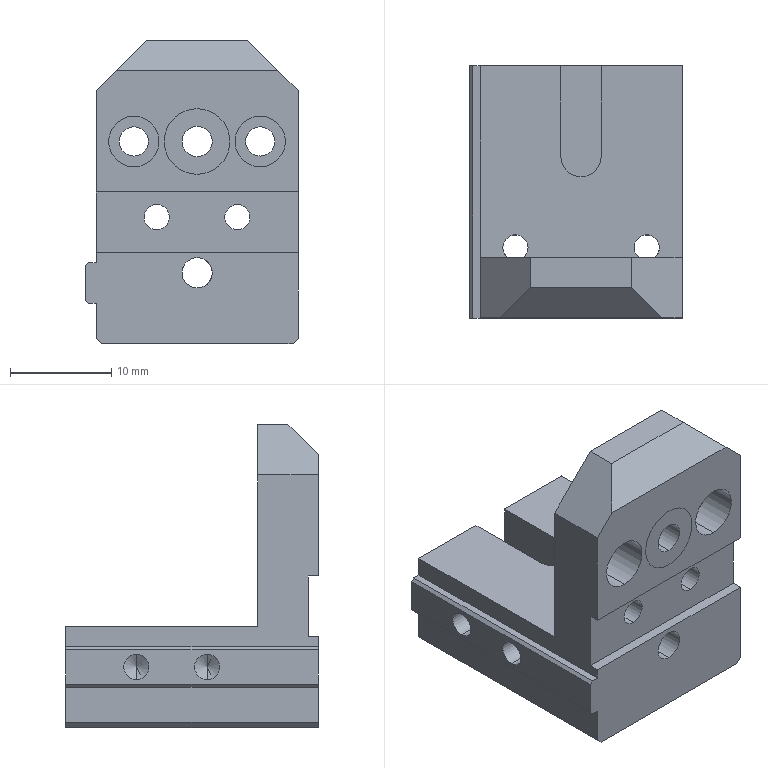Part | SolidWorks | features ICE 7, HoleWzd 6, Chamfer 4, Cut 1, Extrusion 1 | 2 solids | 75 faces | box 21 x 25 x 30 mm | volume 6312 mm3 | cylinder 35 | plane 30 | cone 10 | commonest cylinder face diameters 2.5 x14 2.05 x4 2.9 x4 3 x4 5 x4 6.5 x4